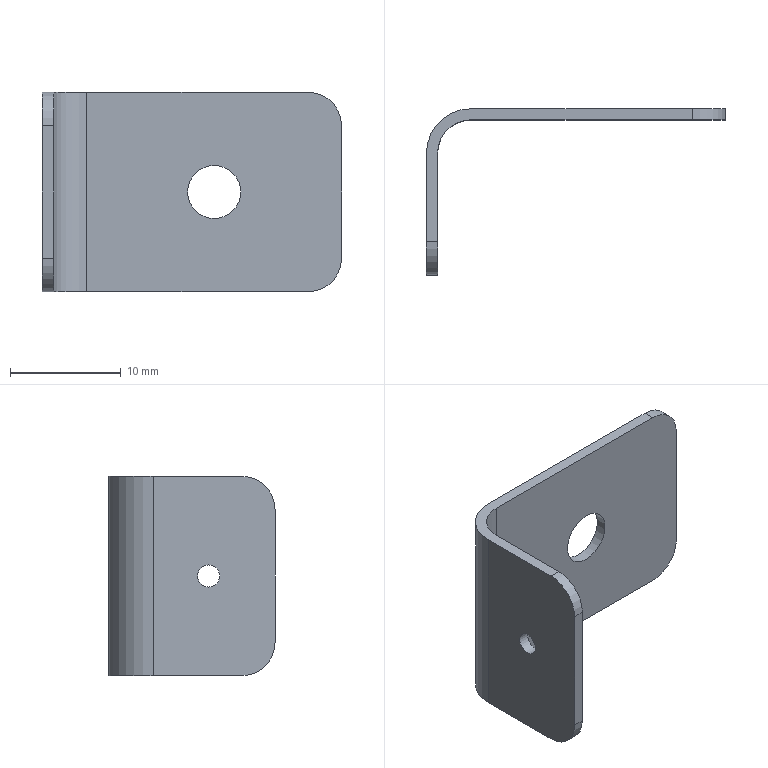Part | NX | features solid 2 | 1 solid | 16 faces | box 27 x 15 x 18 mm | volume 681.997 mm3 | plane 8 | cylinder 8 | commonest cylinder face diameters 6 x5 2 x1 4.8 x1 8 x1
STEP:
#1=CARTESIAN_POINT('',(1.,-9.,10.));
#2=VERTEX_POINT('',#1);
#3=CARTESIAN_POINT('',(1.,-9.,9.));
#4=DIRECTION('',(-1.,0.,0.));
#5=DIRECTION('',(0.,0.,1.));
#6=AXIS2_PLACEMENT_3D('',#3,#4,#5);
#7=CIRCLE('',#6,1.);
#8=EDGE_CURVE('',#2,#2,#7,.T.);
#9=ORIENTED_EDGE('',*,*,#8,.T.);
#10=EDGE_LOOP('',(#9));
#11=FACE_BOUND('',#10,.T.);
#12=CARTESIAN_POINT('',(1.,-15.,15.));
#13=VERTEX_POINT('',#12);
#14=CARTESIAN_POINT('',(1.,-15.,3.));
#15=VERTEX_POINT('',#14);
#16=CARTESIAN_POINT('',(1.,-15.,18.));
#17=DIRECTION('',(0.,0.,-1.));
#18=VECTOR('',#17,1000.);
#19=LINE('',#16,#18);
#20=EDGE_CURVE('',#13,#15,#19,.T.);
#21=ORIENTED_EDGE('',*,*,#20,.T.);
#22=CARTESIAN_POINT('',(1.,-12.,0.));
#23=VERTEX_POINT('',#22);
#24=CARTESIAN_POINT('',(1.,-12.,3.));
#25=DIRECTION('',(1.,0.,0.));
#26=DIRECTION('',(0.,0.,-1.));
#27=AXIS2_PLACEMENT_3D('',#24,#25,#26);
#28=CIRCLE('',#27,3.);
#29=EDGE_CURVE('',#15,#23,#28,.T.);
#30=ORIENTED_EDGE('',*,*,#29,.T.);
#31=CARTESIAN_POINT('',(1.,-4.,0.));
#32=VERTEX_POINT('',#31);
#33=CARTESIAN_POINT('',(1.,-15.,0.));
#34=DIRECTION('',(0.,1.,0.));
#35=VECTOR('',#34,1000.);
#36=LINE('',#33,#35);
#37=EDGE_CURVE('',#23,#32,#36,.T.);
#38=ORIENTED_EDGE('',*,*,#37,.T.);
#39=CARTESIAN_POINT('',(1.,-4.,18.));
#40=VERTEX_POINT('',#39);
#41=CARTESIAN_POINT('',(1.,-4.,18.));
#42=DIRECTION('',(0.,0.,-1.));
#43=VECTOR('',#42,1000.);
#44=LINE('',#41,#43);
#45=EDGE_CURVE('',#32,#40,#44,.F.);
#46=ORIENTED_EDGE('',*,*,#45,.T.);
#47=CARTESIAN_POINT('',(1.,-12.,18.));
#48=VERTEX_POINT('',#47);
#49=CARTESIAN_POINT('',(1.,-15.,18.));
#50=DIRECTION('',(0.,1.,0.));
#51=VECTOR('',#50,1000.);
#52=LINE('',#49,#51);
#53=EDGE_CURVE('',#48,#40,#52,.T.);
#54=ORIENTED_EDGE('',*,*,#53,.F.);
#55=CARTESIAN_POINT('',(1.,-12.,15.));
#56=DIRECTION('',(1.,0.,0.));
#57=DIRECTION('',(0.,0.,-1.));
#58=AXIS2_PLACEMENT_3D('',#55,#56,#57);
#59=CIRCLE('',#58,3.);
#60=EDGE_CURVE('',#48,#13,#59,.T.);
#61=ORIENTED_EDGE('',*,*,#60,.T.);
#62=EDGE_LOOP('',(#21,#30,#38,#46,#54,#61));
#63=FACE_BOUND('',#62,.T.);
#64=CARTESIAN_POINT('',(1.,-15.,18.));
#65=DIRECTION('',(1.,0.,0.));
#66=DIRECTION('',(0.,0.,-1.));
#67=AXIS2_PLACEMENT_3D('',#64,#65,#66);
#68=PLANE('',#67);
#69=ADVANCED_FACE('',(#11,#63),#68,.T.);
#70=CARTESIAN_POINT('',(24.,-1.,18.));
#71=VERTEX_POINT('',#70);
#72=CARTESIAN_POINT('',(4.,-1.,18.));
#73=VERTEX_POINT('',#72);
#74=CARTESIAN_POINT('',(0.,-1.,18.));
#75=DIRECTION('',(1.,0.,0.));
#76=VECTOR('',#75,1000.);
#77=LINE('',#74,#76);
#78=EDGE_CURVE('',#71,#73,#77,.F.);
#79=ORIENTED_EDGE('',*,*,#78,.F.);
#80=CARTESIAN_POINT('',(24.,0.,18.));
#81=VERTEX_POINT('',#80);
#82=CARTESIAN_POINT('',(24.,-15.,18.));
#83=DIRECTION('',(0.,1.,0.));
#84=VECTOR('',#83,1000.);
#85=LINE('',#82,#84);
#86=EDGE_CURVE('',#71,#81,#85,.T.);
#87=ORIENTED_EDGE('',*,*,#86,.T.);
#88=CARTESIAN_POINT('',(4.,0.,18.));
#89=VERTEX_POINT('',#88);
#90=CARTESIAN_POINT('',(27.,0.,18.));
#91=DIRECTION('',(-1.,0.,0.));
#92=VECTOR('',#91,1000.);
#93=LINE('',#90,#92);
#94=EDGE_CURVE('',#81,#89,#93,.T.);
#95=ORIENTED_EDGE('',*,*,#94,.T.);
#96=CARTESIAN_POINT('',(0.,-4.,18.));
#97=VERTEX_POINT('',#96);
#98=CARTESIAN_POINT('',(4.,-4.,18.));
#99=DIRECTION('',(0.,0.,-1.));
#100=DIRECTION('',(1.,0.,0.));
#101=AXIS2_PLACEMENT_3D('',#98,#99,#100);
#102=CIRCLE('',#101,4.);
#103=EDGE_CURVE('',#97,#89,#102,.T.);
#104=ORIENTED_EDGE('',*,*,#103,.F.);
#105=CARTESIAN_POINT('',(0.,-12.,18.));
#106=VERTEX_POINT('',#105);
#107=CARTESIAN_POINT('',(0.,-15.,18.));
#108=DIRECTION('',(0.,1.,0.));
#109=VECTOR('',#108,1000.);
#110=LINE('',#107,#109);
#111=EDGE_CURVE('',#106,#97,#110,.T.);
#112=ORIENTED_EDGE('',*,*,#111,.F.);
#113=CARTESIAN_POINT('',(0.,-12.,18.));
#114=DIRECTION('',(-1.,0.,0.));
#115=VECTOR('',#114,1000.);
#116=LINE('',#113,#115);
#117=EDGE_CURVE('',#106,#48,#116,.F.);
#118=ORIENTED_EDGE('',*,*,#117,.T.);
#119=ORIENTED_EDGE('',*,*,#53,.T.);
#120=CARTESIAN_POINT('',(4.,-4.,18.));
#121=DIRECTION('',(0.,0.,-1.));
#122=DIRECTION('',(-1.,0.,0.));
#123=AXIS2_PLACEMENT_3D('',#120,#121,#122);
#124=CIRCLE('',#123,3.);
#125=EDGE_CURVE('',#40,#73,#124,.T.);
#126=ORIENTED_EDGE('',*,*,#125,.T.);
#127=EDGE_LOOP('',(#79,#87,#95,#104,#112,#118,#119,#126));
#128=FACE_BOUND('',#127,.T.);
#129=CARTESIAN_POINT('',(0.,-15.,18.));
#130=DIRECTION('',(0.,0.,-1.));
#131=DIRECTION('',(0.,1.,0.));
#132=AXIS2_PLACEMENT_3D('',#129,#130,#131);
#133=PLANE('',#132);
#134=ADVANCED_FACE('',(#128),#133,.F.);
#135=CARTESIAN_POINT('',(4.,0.,0.));
#136=VERTEX_POINT('',#135);
#137=CARTESIAN_POINT('',(24.,0.,0.));
#138=VERTEX_POINT('',#137);
#139=CARTESIAN_POINT('',(0.,0.,0.));
#140=DIRECTION('',(1.,0.,0.));
#141=VECTOR('',#140,1000.);
#142=LINE('',#139,#141);
#143=EDGE_CURVE('',#136,#138,#142,.T.);
#144=ORIENTED_EDGE('',*,*,#143,.T.);
#145=CARTESIAN_POINT('',(24.,-1.,0.));
#146=VERTEX_POINT('',#145);
#147=CARTESIAN_POINT('',(24.,-15.,0.));
#148=DIRECTION('',(0.,1.,0.));
#149=VECTOR('',#148,1000.);
#150=LINE('',#147,#149);
#151=EDGE_CURVE('',#138,#146,#150,.F.);
#152=ORIENTED_EDGE('',*,*,#151,.T.);
#153=CARTESIAN_POINT('',(4.,-1.,0.));
#154=VERTEX_POINT('',#153);
#155=CARTESIAN_POINT('',(0.,-1.,0.));
#156=DIRECTION('',(1.,0.,0.));
#157=VECTOR('',#156,1000.);
#158=LINE('',#155,#157);
#159=EDGE_CURVE('',#154,#146,#158,.T.);
#160=ORIENTED_EDGE('',*,*,#159,.F.);
#161=CARTESIAN_POINT('',(4.,-4.,0.));
#162=DIRECTION('',(0.,0.,-1.));
#163=DIRECTION('',(-1.,0.,0.));
#164=AXIS2_PLACEMENT_3D('',#161,#162,#163);
#165=CIRCLE('',#164,3.);
#166=EDGE_CURVE('',#32,#154,#165,.T.);
#167=ORIENTED_EDGE('',*,*,#166,.F.);
#168=ORIENTED_EDGE('',*,*,#37,.F.);
#169=CARTESIAN_POINT('',(0.,-12.,0.));
#170=VERTEX_POINT('',#169);
#171=CARTESIAN_POINT('',(0.,-12.,0.));
#172=DIRECTION('',(-1.,0.,0.));
#173=VECTOR('',#172,1000.);
#174=LINE('',#171,#173);
#175=EDGE_CURVE('',#23,#170,#174,.T.);
#176=ORIENTED_EDGE('',*,*,#175,.T.);
#177=CARTESIAN_POINT('',(0.,-4.,0.));
#178=VERTEX_POINT('',#177);
#179=CARTESIAN_POINT('',(0.,-15.,0.));
#180=DIRECTION('',(0.,1.,0.));
#181=VECTOR('',#180,1000.);
#182=LINE('',#179,#181);
#183=EDGE_CURVE('',#170,#178,#182,.T.);
#184=ORIENTED_EDGE('',*,*,#183,.T.);
#185=CARTESIAN_POINT('',(4.,-4.,0.));
#186=DIRECTION('',(0.,0.,-1.));
#187=DIRECTION('',(1.,0.,0.));
#188=AXIS2_PLACEMENT_3D('',#185,#186,#187);
#189=CIRCLE('',#188,4.);
#190=EDGE_CURVE('',#178,#136,#189,.T.);
#191=ORIENTED_EDGE('',*,*,#190,.T.);
#192=EDGE_LOOP('',(#144,#152,#160,#167,#168,#176,#184,#191));
#193=FACE_BOUND('',#192,.T.);
#194=CARTESIAN_POINT('',(0.,-15.,0.));
#195=DIRECTION('',(0.,0.,-1.));
#196=DIRECTION('',(0.,1.,0.));
#197=AXIS2_PLACEMENT_3D('',#194,#195,#196);
#198=PLANE('',#197);
#199=ADVANCED_FACE('',(#193),#198,.T.);
#200=CARTESIAN_POINT('',(0.,-9.,8.));
#201=VERTEX_POINT('',#200);
#202=CARTESIAN_POINT('',(0.,-9.,9.));
#203=DIRECTION('',(1.,0.,0.));
#204=DIRECTION('',(0.,0.,-1.));
#205=AXIS2_PLACEMENT_3D('',#202,#203,#204);
#206=CIRCLE('',#205,1.);
#207=EDGE_CURVE('',#201,#201,#206,.T.);
#208=ORIENTED_EDGE('',*,*,#207,.T.);
#209=EDGE_LOOP('',(#208));
#210=FACE_BOUND('',#209,.T.);
#211=ORIENTED_EDGE('',*,*,#183,.F.);
#212=CARTESIAN_POINT('',(0.,-15.,3.));
#213=VERTEX_POINT('',#212);
#214=CARTESIAN_POINT('',(0.,-12.,3.));
#215=DIRECTION('',(1.,0.,0.));
#216=DIRECTION('',(0.,0.,-1.));
#217=AXIS2_PLACEMENT_3D('',#214,#215,#216);
#218=CIRCLE('',#217,3.);
#219=EDGE_CURVE('',#170,#213,#218,.F.);
#220=ORIENTED_EDGE('',*,*,#219,.T.);
#221=CARTESIAN_POINT('',(0.,-15.,15.));
#222=VERTEX_POINT('',#221);
#223=CARTESIAN_POINT('',(0.,-15.,18.));
#224=DIRECTION('',(0.,0.,-1.));
#225=VECTOR('',#224,1000.);
#226=LINE('',#223,#225);
#227=EDGE_CURVE('',#222,#213,#226,.T.);
#228=ORIENTED_EDGE('',*,*,#227,.F.);
#229=CARTESIAN_POINT('',(0.,-12.,15.));
#230=DIRECTION('',(1.,0.,0.));
#231=DIRECTION('',(0.,0.,-1.));
#232=AXIS2_PLACEMENT_3D('',#229,#230,#231);
#233=CIRCLE('',#232,3.);
#234=EDGE_CURVE('',#222,#106,#233,.F.);
#235=ORIENTED_EDGE('',*,*,#234,.T.);
#236=ORIENTED_EDGE('',*,*,#111,.T.);
#237=CARTESIAN_POINT('',(0.,-4.,0.));
#238=DIRECTION('',(0.,0.,1.));
#239=VECTOR('',#238,1000.);
#240=LINE('',#237,#239);
#241=EDGE_CURVE('',#178,#97,#240,.T.);
#242=ORIENTED_EDGE('',*,*,#241,.F.);
#243=EDGE_LOOP('',(#211,#220,#228,#235,#236,#242));
#244=FACE_BOUND('',#243,.T.);
#245=CARTESIAN_POINT('',(0.,-15.,18.));
#246=DIRECTION('',(1.,0.,0.));
#247=DIRECTION('',(0.,0.,-1.));
#248=AXIS2_PLACEMENT_3D('',#245,#246,#247);
#249=PLANE('',#248);
#250=ADVANCED_FACE('',(#210,#244),#249,.F.);
#251=ORIENTED_EDGE('',*,*,#227,.T.);
#252=CARTESIAN_POINT('',(0.,-15.,3.));
#253=DIRECTION('',(-1.,0.,0.));
#254=VECTOR('',#253,1000.);
#255=LINE('',#252,#254);
#256=EDGE_CURVE('',#213,#15,#255,.F.);
#257=ORIENTED_EDGE('',*,*,#256,.T.);
#258=ORIENTED_EDGE('',*,*,#20,.F.);
#259=CARTESIAN_POINT('',(0.,-15.,15.));
#260=DIRECTION('',(1.,0.,0.));
#261=VECTOR('',#260,1000.);
#262=LINE('',#259,#261);
#263=EDGE_CURVE('',#13,#222,#262,.F.);
#264=ORIENTED_EDGE('',*,*,#263,.T.);
#265=EDGE_LOOP('',(#251,#257,#258,#264));
#266=FACE_BOUND('',#265,.T.);
#267=CARTESIAN_POINT('',(0.,-15.,18.));
#268=DIRECTION('',(0.,-1.,0.));
#269=DIRECTION('',(0.,0.,-1.));
#270=AXIS2_PLACEMENT_3D('',#267,#268,#269);
#271=PLANE('',#270);
#272=ADVANCED_FACE('',(#266),#271,.T.);
#273=CARTESIAN_POINT('',(27.,-1.,3.));
#274=VERTEX_POINT('',#273);
#275=CARTESIAN_POINT('',(27.,-1.,15.));
#276=VERTEX_POINT('',#275);
#277=CARTESIAN_POINT('',(27.,-1.,0.));
#278=DIRECTION('',(0.,0.,-1.));
#279=VECTOR('',#278,1000.);
#280=LINE('',#277,#279);
#281=EDGE_CURVE('',#274,#276,#280,.F.);
#282=ORIENTED_EDGE('',*,*,#281,.F.);
#283=CARTESIAN_POINT('',(27.,0.,3.));
#284=VERTEX_POINT('',#283);
#285=CARTESIAN_POINT('',(27.,0.,3.));
#286=DIRECTION('',(0.,1.,0.));
#287=VECTOR('',#286,1000.);
#288=LINE('',#285,#287);
#289=EDGE_CURVE('',#274,#284,#288,.T.);
#290=ORIENTED_EDGE('',*,*,#289,.T.);
#291=CARTESIAN_POINT('',(27.,0.,15.));
#292=VERTEX_POINT('',#291);
#293=CARTESIAN_POINT('',(27.,0.,0.));
#294=DIRECTION('',(0.,0.,1.));
#295=VECTOR('',#294,1000.);
#296=LINE('',#293,#295);
#297=EDGE_CURVE('',#284,#292,#296,.T.);
#298=ORIENTED_EDGE('',*,*,#297,.T.);
#299=CARTESIAN_POINT('',(27.,0.,15.));
#300=DIRECTION('',(0.,-1.,0.));
#301=VECTOR('',#300,1000.);
#302=LINE('',#299,#301);
#303=EDGE_CURVE('',#292,#276,#302,.T.);
#304=ORIENTED_EDGE('',*,*,#303,.T.);
#305=EDGE_LOOP('',(#282,#290,#298,#304));
#306=FACE_BOUND('',#305,.T.);
#307=CARTESIAN_POINT('',(27.,0.,0.));
#308=DIRECTION('',(1.,0.,0.));
#309=DIRECTION('',(0.,0.,1.));
#310=AXIS2_PLACEMENT_3D('',#307,#308,#309);
#311=PLANE('',#310);
#312=ADVANCED_FACE('',(#306),#311,.T.);
#313=CARTESIAN_POINT('',(15.5,-1.,11.4));
#314=VERTEX_POINT('',#313);
#315=CARTESIAN_POINT('',(15.5,-1.,9.));
#316=DIRECTION('',(0.,1.,0.));
#317=DIRECTION('',(0.,0.,1.));
#318=AXIS2_PLACEMENT_3D('',#315,#316,#317);
#319=CIRCLE('',#318,2.4);
#320=EDGE_CURVE('',#314,#314,#319,.T.);
#321=ORIENTED_EDGE('',*,*,#320,.T.);
#322=EDGE_LOOP('',(#321));
#323=FACE_BOUND('',#322,.T.);
#324=ORIENTED_EDGE('',*,*,#159,.T.);
#325=CARTESIAN_POINT('',(24.,-1.,3.));
#326=DIRECTION('',(0.,-1.,0.));
#327=DIRECTION('',(0.,0.,-1.));
#328=AXIS2_PLACEMENT_3D('',#325,#326,#327);
#329=CIRCLE('',#328,3.);
#330=EDGE_CURVE('',#146,#274,#329,.T.);
#331=ORIENTED_EDGE('',*,*,#330,.T.);
#332=ORIENTED_EDGE('',*,*,#281,.T.);
#333=CARTESIAN_POINT('',(24.,-1.,15.));
#334=DIRECTION('',(0.,-1.,0.));
#335=DIRECTION('',(0.,0.,-1.));
#336=AXIS2_PLACEMENT_3D('',#333,#334,#335);
#337=CIRCLE('',#336,3.);
#338=EDGE_CURVE('',#276,#71,#337,.T.);
#339=ORIENTED_EDGE('',*,*,#338,.T.);
#340=ORIENTED_EDGE('',*,*,#78,.T.);
#341=CARTESIAN_POINT('',(4.,-1.,18.));
#342=DIRECTION('',(0.,0.,-1.));
#343=VECTOR('',#342,1000.);
#344=LINE('',#341,#343);
#345=EDGE_CURVE('',#154,#73,#344,.F.);
#346=ORIENTED_EDGE('',*,*,#345,.F.);
#347=EDGE_LOOP('',(#324,#331,#332,#339,#340,#346));
#348=FACE_BOUND('',#347,.T.);
#349=CARTESIAN_POINT('',(0.,-1.,0.));
#350=DIRECTION('',(0.,-1.,0.));
#351=DIRECTION('',(0.,0.,-1.));
#352=AXIS2_PLACEMENT_3D('',#349,#350,#351);
#353=PLANE('',#352);
#354=ADVANCED_FACE('',(#323,#348),#353,.T.);
#355=CARTESIAN_POINT('',(15.5,0.,6.6));
#356=VERTEX_POINT('',#355);
#357=CARTESIAN_POINT('',(15.5,0.,9.));
#358=DIRECTION('',(0.,-1.,0.));
#359=DIRECTION('',(0.,0.,-1.));
#360=AXIS2_PLACEMENT_3D('',#357,#358,#359);
#361=CIRCLE('',#360,2.4);
#362=EDGE_CURVE('',#356,#356,#361,.T.);
#363=ORIENTED_EDGE('',*,*,#362,.T.);
#364=EDGE_LOOP('',(#363));
#365=FACE_BOUND('',#364,.T.);
#366=ORIENTED_EDGE('',*,*,#297,.F.);
#367=CARTESIAN_POINT('',(24.,0.,3.));
#368=DIRECTION('',(0.,-1.,0.));
#369=DIRECTION('',(0.,0.,-1.));
#370=AXIS2_PLACEMENT_3D('',#367,#368,#369);
#371=CIRCLE('',#370,3.);
#372=EDGE_CURVE('',#284,#138,#371,.F.);
#373=ORIENTED_EDGE('',*,*,#372,.T.);
#374=ORIENTED_EDGE('',*,*,#143,.F.);
#375=CARTESIAN_POINT('',(4.,0.,0.));
#376=DIRECTION('',(0.,0.,1.));
#377=VECTOR('',#376,1000.);
#378=LINE('',#375,#377);
#379=EDGE_CURVE('',#136,#89,#378,.T.);
#380=ORIENTED_EDGE('',*,*,#379,.T.);
#381=ORIENTED_EDGE('',*,*,#94,.F.);
#382=CARTESIAN_POINT('',(24.,0.,15.));
#383=DIRECTION('',(0.,-1.,0.));
#384=DIRECTION('',(0.,0.,-1.));
#385=AXIS2_PLACEMENT_3D('',#382,#383,#384);
#386=CIRCLE('',#385,3.);
#387=EDGE_CURVE('',#81,#292,#386,.F.);
#388=ORIENTED_EDGE('',*,*,#387,.T.);
#389=EDGE_LOOP('',(#366,#373,#374,#380,#381,#388));
#390=FACE_BOUND('',#389,.T.);
#391=CARTESIAN_POINT('',(0.,0.,0.));
#392=DIRECTION('',(0.,-1.,0.));
#393=DIRECTION('',(0.,0.,-1.));
#394=AXIS2_PLACEMENT_3D('',#391,#392,#393);
#395=PLANE('',#394);
#396=ADVANCED_FACE('',(#365,#390),#395,.F.);
#397=ORIENTED_EDGE('',*,*,#379,.F.);
#398=ORIENTED_EDGE('',*,*,#190,.F.);
#399=ORIENTED_EDGE('',*,*,#241,.T.);
#400=ORIENTED_EDGE('',*,*,#103,.T.);
#401=EDGE_LOOP('',(#397,#398,#399,#400));
#402=FACE_BOUND('',#401,.T.);
#403=CARTESIAN_POINT('',(4.,-4.,18.));
#404=DIRECTION('',(0.,0.,-1.));
#405=DIRECTION('',(1.,0.,0.));
#406=AXIS2_PLACEMENT_3D('',#403,#404,#405);
#407=CYLINDRICAL_SURFACE('',#406,4.);
#408=ADVANCED_FACE('',(#402),#407,.T.);
#409=ORIENTED_EDGE('',*,*,#345,.T.);
#410=ORIENTED_EDGE('',*,*,#125,.F.);
#411=ORIENTED_EDGE('',*,*,#45,.F.);
#412=ORIENTED_EDGE('',*,*,#166,.T.);
#413=EDGE_LOOP('',(#409,#410,#411,#412));
#414=FACE_BOUND('',#413,.T.);
#415=CARTESIAN_POINT('',(4.,-4.,18.));
#416=DIRECTION('',(0.,0.,-1.));
#417=DIRECTION('',(1.,0.,0.));
#418=AXIS2_PLACEMENT_3D('',#415,#416,#417);
#419=CYLINDRICAL_SURFACE('',#418,3.);
#420=ADVANCED_FACE('',(#414),#419,.F.);
#421=ORIENTED_EDGE('',*,*,#320,.F.);
#422=EDGE_LOOP('',(#421));
#423=FACE_BOUND('',#422,.T.);
#424=ORIENTED_EDGE('',*,*,#362,.F.);
#425=EDGE_LOOP('',(#424));
#426=FACE_BOUND('',#425,.T.);
#427=CARTESIAN_POINT('',(15.5,-1.,9.));
#428=DIRECTION('',(0.,1.,0.));
#429=DIRECTION('',(0.,0.,1.));
#430=AXIS2_PLACEMENT_3D('',#427,#428,#429);
#431=CYLINDRICAL_SURFACE('',#430,2.4);
#432=ADVANCED_FACE('',(#423,#426),#431,.F.);
#433=ORIENTED_EDGE('',*,*,#8,.F.);
#434=EDGE_LOOP('',(#433));
#435=FACE_BOUND('',#434,.T.);
#436=ORIENTED_EDGE('',*,*,#207,.F.);
#437=EDGE_LOOP('',(#436));
#438=FACE_BOUND('',#437,.T.);
#439=CARTESIAN_POINT('',(1.,-9.,9.));
#440=DIRECTION('',(-1.,0.,0.));
#441=DIRECTION('',(0.,0.,1.));
#442=AXIS2_PLACEMENT_3D('',#439,#440,#441);
#443=CYLINDRICAL_SURFACE('',#442,1.);
#444=ADVANCED_FACE('',(#435,#438),#443,.F.);
#445=ORIENTED_EDGE('',*,*,#372,.F.);
#446=ORIENTED_EDGE('',*,*,#289,.F.);
#447=ORIENTED_EDGE('',*,*,#330,.F.);
#448=ORIENTED_EDGE('',*,*,#151,.F.);
#449=EDGE_LOOP('',(#445,#446,#447,#448));
#450=FACE_BOUND('',#449,.T.);
#451=CARTESIAN_POINT('',(24.,-15.,3.));
#452=DIRECTION('',(0.,-1.,0.));
#453=DIRECTION('',(0.,0.,-1.));
#454=AXIS2_PLACEMENT_3D('',#451,#452,#453);
#455=CYLINDRICAL_SURFACE('',#454,3.);
#456=ADVANCED_FACE('',(#450),#455,.T.);
#457=ORIENTED_EDGE('',*,*,#387,.F.);
#458=ORIENTED_EDGE('',*,*,#86,.F.);
#459=ORIENTED_EDGE('',*,*,#338,.F.);
#460=ORIENTED_EDGE('',*,*,#303,.F.);
#461=EDGE_LOOP('',(#457,#458,#459,#460));
#462=FACE_BOUND('',#461,.T.);
#463=CARTESIAN_POINT('',(24.,0.,15.));
#464=DIRECTION('',(0.,1.,0.));
#465=DIRECTION('',(0.,0.,1.));
#466=AXIS2_PLACEMENT_3D('',#463,#464,#465);
#467=CYLINDRICAL_SURFACE('',#466,3.);
#468=ADVANCED_FACE('',(#462),#467,.T.);
#469=ORIENTED_EDGE('',*,*,#219,.F.);
#470=ORIENTED_EDGE('',*,*,#175,.F.);
#471=ORIENTED_EDGE('',*,*,#29,.F.);
#472=ORIENTED_EDGE('',*,*,#256,.F.);
#473=EDGE_LOOP('',(#469,#470,#471,#472));
#474=FACE_BOUND('',#473,.T.);
#475=CARTESIAN_POINT('',(0.,-12.,3.));
#476=DIRECTION('',(1.,0.,0.));
#477=DIRECTION('',(0.,0.,-1.));
#478=AXIS2_PLACEMENT_3D('',#475,#476,#477);
#479=CYLINDRICAL_SURFACE('',#478,3.);
#480=ADVANCED_FACE('',(#474),#479,.T.);
#481=ORIENTED_EDGE('',*,*,#234,.F.);
#482=ORIENTED_EDGE('',*,*,#263,.F.);
#483=ORIENTED_EDGE('',*,*,#60,.F.);
#484=ORIENTED_EDGE('',*,*,#117,.F.);
#485=EDGE_LOOP('',(#481,#482,#483,#484));
#486=FACE_BOUND('',#485,.T.);
#487=CARTESIAN_POINT('',(0.,-12.,15.));
#488=DIRECTION('',(-1.,0.,0.));
#489=DIRECTION('',(0.,0.,1.));
#490=AXIS2_PLACEMENT_3D('',#487,#488,#489);
#491=CYLINDRICAL_SURFACE('',#490,3.);
#492=ADVANCED_FACE('',(#486),#491,.T.);
#493=CLOSED_SHELL('',(#69,#134,#199,#250,#272,#312,#354,#396,#408,#420,#432,#444,#456,#468,#480,#492));
#494=MANIFOLD_SOLID_BREP('',#493);
#495=(LENGTH_UNIT()NAMED_UNIT(*)SI_UNIT(.MILLI.,.METRE.));
#496=UNCERTAINTY_MEASURE_WITH_UNIT(LENGTH_MEASURE(0.00001),#495,'','');
#497=(NAMED_UNIT(*)PLANE_ANGLE_UNIT()SI_UNIT($,.RADIAN.));
#498=(NAMED_UNIT(*)SI_UNIT($,.STERADIAN.)SOLID_ANGLE_UNIT());
#499=(GEOMETRIC_REPRESENTATION_CONTEXT(3)GLOBAL_UNCERTAINTY_ASSIGNED_CONTEXT((#496))GLOBAL_UNIT_ASSIGNED_CONTEXT((#495,#497,#498))REPRESENTATION_CONTEXT('',''));
#500=ADVANCED_BREP_SHAPE_REPRESENTATION('',(#494),#499);